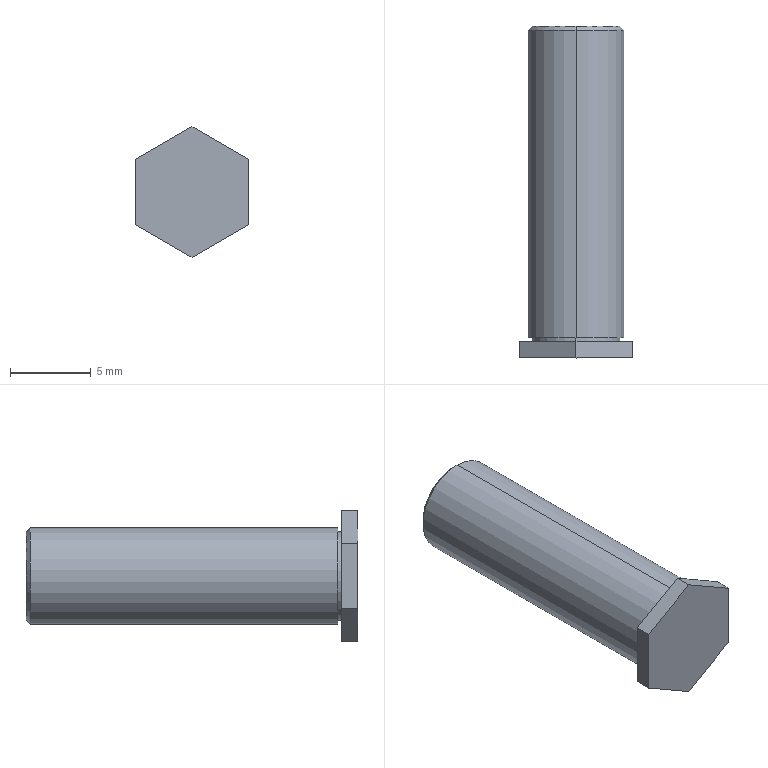Part | NX | features BREP 1 | 1 solid | 21 faces | box 7 x 20.5 x 8.083 mm | volume 432.929 mm3 | plane 11 | cylinder 6 | cone 4 | commonest cylinder face diameters 3.3 x2 5.45 x2 5.95 x2
STEP:
#1=CARTESIAN_POINT('',(300.5,41.65,424.025));
#2=VERTEX_POINT('',#1);
#3=CARTESIAN_POINT('',(300.5,41.65,429.975));
#4=VERTEX_POINT('',#3);
#5=CARTESIAN_POINT('',(300.5,41.65,427.));
#6=DIRECTION('',(0.,-1.,0.));
#7=DIRECTION('',(0.,0.,-1.));
#8=AXIS2_PLACEMENT_3D('',#5,#6,#7);
#9=CIRCLE('',#8,2.975);
#10=EDGE_CURVE('',#2,#4,#9,.T.);
#11=ORIENTED_EDGE('',*,*,#10,.T.);
#12=CARTESIAN_POINT('',(300.5,22.65,429.975));
#13=VERTEX_POINT('',#12);
#14=CARTESIAN_POINT('',(300.5,31.4,429.975));
#15=DIRECTION('',(0.,-1.,0.));
#16=VECTOR('',#15,1000.);
#17=LINE('',#14,#16);
#18=EDGE_CURVE('',#13,#4,#17,.F.);
#19=ORIENTED_EDGE('',*,*,#18,.F.);
#20=CARTESIAN_POINT('',(300.5,22.65,424.025));
#21=VERTEX_POINT('',#20);
#22=CARTESIAN_POINT('',(300.5,22.65,427.));
#23=DIRECTION('',(0.,1.,0.));
#24=DIRECTION('',(0.,0.,-1.));
#25=AXIS2_PLACEMENT_3D('',#22,#23,#24);
#26=CIRCLE('',#25,2.975);
#27=EDGE_CURVE('',#13,#21,#26,.T.);
#28=ORIENTED_EDGE('',*,*,#27,.T.);
#29=CARTESIAN_POINT('',(300.5,31.4,424.025));
#30=DIRECTION('',(0.,-1.,0.));
#31=VECTOR('',#30,1000.);
#32=LINE('',#29,#31);
#33=EDGE_CURVE('',#21,#2,#32,.F.);
#34=ORIENTED_EDGE('',*,*,#33,.T.);
#35=EDGE_LOOP('',(#11,#19,#28,#34));
#36=FACE_BOUND('',#35,.T.);
#37=CARTESIAN_POINT('',(300.5,31.4,427.));
#38=DIRECTION('',(0.,-1.,0.));
#39=DIRECTION('',(0.,0.,1.));
#40=AXIS2_PLACEMENT_3D('',#37,#38,#39);
#41=CYLINDRICAL_SURFACE('',#40,2.975);
#42=ADVANCED_FACE('',(#36),#41,.T.);
#43=CARTESIAN_POINT('',(300.5,41.9,424.275));
#44=VERTEX_POINT('',#43);
#45=CARTESIAN_POINT('',(300.5,41.9,429.725));
#46=VERTEX_POINT('',#45);
#47=CARTESIAN_POINT('',(300.5,41.9,427.));
#48=DIRECTION('',(0.,-1.,0.));
#49=DIRECTION('',(0.,0.,-1.));
#50=AXIS2_PLACEMENT_3D('',#47,#48,#49);
#51=CIRCLE('',#50,2.725);
#52=EDGE_CURVE('',#44,#46,#51,.T.);
#53=ORIENTED_EDGE('',*,*,#52,.T.);
#54=CARTESIAN_POINT('',(300.5,41.65,429.975));
#55=DIRECTION('',(0.,-0.7071,0.7071));
#56=VECTOR('',#55,1000.);
#57=LINE('',#54,#56);
#58=EDGE_CURVE('',#4,#46,#57,.F.);
#59=ORIENTED_EDGE('',*,*,#58,.F.);
#60=ORIENTED_EDGE('',*,*,#10,.F.);
#61=CARTESIAN_POINT('',(300.5,41.65,424.025));
#62=DIRECTION('',(0.,-0.7071,-0.7071));
#63=VECTOR('',#62,1000.);
#64=LINE('',#61,#63);
#65=EDGE_CURVE('',#2,#44,#64,.F.);
#66=ORIENTED_EDGE('',*,*,#65,.T.);
#67=EDGE_LOOP('',(#53,#59,#60,#66));
#68=FACE_BOUND('',#67,.T.);
#69=CARTESIAN_POINT('',(300.5,41.65,427.));
#70=DIRECTION('',(0.,-1.,0.));
#71=DIRECTION('',(0.,0.,1.));
#72=AXIS2_PLACEMENT_3D('',#69,#70,#71);
#73=CONICAL_SURFACE('',#72,2.975,0.7854);
#74=ADVANCED_FACE('',(#68),#73,.T.);
#75=CARTESIAN_POINT('',(300.5,22.4,429.725));
#76=VERTEX_POINT('',#75);
#77=CARTESIAN_POINT('',(300.5,22.4,424.275));
#78=VERTEX_POINT('',#77);
#79=CARTESIAN_POINT('',(300.5,22.4,427.));
#80=DIRECTION('',(0.,1.,0.));
#81=DIRECTION('',(0.,0.,1.));
#82=AXIS2_PLACEMENT_3D('',#79,#80,#81);
#83=CIRCLE('',#82,2.725);
#84=EDGE_CURVE('',#76,#78,#83,.T.);
#85=ORIENTED_EDGE('',*,*,#84,.T.);
#86=CARTESIAN_POINT('',(300.5,22.65,424.275));
#87=VERTEX_POINT('',#86);
#88=CARTESIAN_POINT('',(300.5,-1.133,424.275));
#89=DIRECTION('',(0.,1.,0.));
#90=VECTOR('',#89,1000.);
#91=LINE('',#88,#90);
#92=EDGE_CURVE('',#78,#87,#91,.T.);
#93=ORIENTED_EDGE('',*,*,#92,.T.);
#94=CARTESIAN_POINT('',(300.5,22.65,429.725));
#95=VERTEX_POINT('',#94);
#96=CARTESIAN_POINT('',(300.5,22.65,427.));
#97=DIRECTION('',(0.,-1.,0.));
#98=DIRECTION('',(0.,0.,1.));
#99=AXIS2_PLACEMENT_3D('',#96,#97,#98);
#100=CIRCLE('',#99,2.725);
#101=EDGE_CURVE('',#87,#95,#100,.T.);
#102=ORIENTED_EDGE('',*,*,#101,.T.);
#103=CARTESIAN_POINT('',(300.5,-1.133,429.725));
#104=DIRECTION('',(0.,1.,0.));
#105=VECTOR('',#104,1000.);
#106=LINE('',#103,#105);
#107=EDGE_CURVE('',#76,#95,#106,.T.);
#108=ORIENTED_EDGE('',*,*,#107,.F.);
#109=EDGE_LOOP('',(#85,#93,#102,#108));
#110=FACE_BOUND('',#109,.T.);
#111=CARTESIAN_POINT('',(300.5,-1.133,427.));
#112=DIRECTION('',(0.,1.,0.));
#113=DIRECTION('',(0.,0.,-1.));
#114=AXIS2_PLACEMENT_3D('',#111,#112,#113);
#115=CYLINDRICAL_SURFACE('',#114,2.725);
#116=ADVANCED_FACE('',(#110),#115,.T.);
#117=CARTESIAN_POINT('',(300.5,41.65,425.35));
#118=VERTEX_POINT('',#117);
#119=CARTESIAN_POINT('',(300.5,41.65,428.65));
#120=VERTEX_POINT('',#119);
#121=CARTESIAN_POINT('',(300.5,41.65,427.));
#122=DIRECTION('',(0.,1.,0.));
#123=DIRECTION('',(0.,0.,1.));
#124=AXIS2_PLACEMENT_3D('',#121,#122,#123);
#125=CIRCLE('',#124,1.65);
#126=EDGE_CURVE('',#118,#120,#125,.T.);
#127=ORIENTED_EDGE('',*,*,#126,.F.);
#128=CARTESIAN_POINT('',(300.5,41.9,425.1));
#129=VERTEX_POINT('',#128);
#130=CARTESIAN_POINT('',(300.5,41.9,425.1));
#131=DIRECTION('',(0.,0.7071,-0.7071));
#132=VECTOR('',#131,1000.);
#133=LINE('',#130,#132);
#134=EDGE_CURVE('',#118,#129,#133,.T.);
#135=ORIENTED_EDGE('',*,*,#134,.T.);
#136=CARTESIAN_POINT('',(300.5,41.9,428.9));
#137=VERTEX_POINT('',#136);
#138=CARTESIAN_POINT('',(300.5,41.9,427.));
#139=DIRECTION('',(0.,-1.,0.));
#140=DIRECTION('',(0.,0.,1.));
#141=AXIS2_PLACEMENT_3D('',#138,#139,#140);
#142=CIRCLE('',#141,1.9);
#143=EDGE_CURVE('',#137,#129,#142,.T.);
#144=ORIENTED_EDGE('',*,*,#143,.F.);
#145=CARTESIAN_POINT('',(300.5,41.9,428.9));
#146=DIRECTION('',(0.,0.7071,0.7071));
#147=VECTOR('',#146,1000.);
#148=LINE('',#145,#147);
#149=EDGE_CURVE('',#120,#137,#148,.T.);
#150=ORIENTED_EDGE('',*,*,#149,.F.);
#151=EDGE_LOOP('',(#127,#135,#144,#150));
#152=FACE_BOUND('',#151,.T.);
#153=CARTESIAN_POINT('',(300.5,41.9,427.));
#154=DIRECTION('',(0.,1.,0.));
#155=DIRECTION('',(0.,0.,-1.));
#156=AXIS2_PLACEMENT_3D('',#153,#154,#155);
#157=CONICAL_SURFACE('',#156,1.9,0.7854);
#158=ADVANCED_FACE('',(#152),#157,.F.);
#159=CARTESIAN_POINT('',(300.5,24.4,425.35));
#160=VERTEX_POINT('',#159);
#161=CARTESIAN_POINT('',(300.5,24.4,428.65));
#162=VERTEX_POINT('',#161);
#163=CARTESIAN_POINT('',(300.5,24.4,427.));
#164=DIRECTION('',(0.,1.,0.));
#165=DIRECTION('',(0.,0.,1.));
#166=AXIS2_PLACEMENT_3D('',#163,#164,#165);
#167=CIRCLE('',#166,1.65);
#168=EDGE_CURVE('',#160,#162,#167,.T.);
#169=ORIENTED_EDGE('',*,*,#168,.F.);
#170=CARTESIAN_POINT('',(300.5,24.4,425.35));
#171=DIRECTION('',(0.,1.,0.));
#172=VECTOR('',#171,1000.);
#173=LINE('',#170,#172);
#174=EDGE_CURVE('',#160,#118,#173,.T.);
#175=ORIENTED_EDGE('',*,*,#174,.T.);
#176=ORIENTED_EDGE('',*,*,#126,.T.);
#177=CARTESIAN_POINT('',(300.5,24.4,428.65));
#178=DIRECTION('',(0.,1.,0.));
#179=VECTOR('',#178,1000.);
#180=LINE('',#177,#179);
#181=EDGE_CURVE('',#162,#120,#180,.T.);
#182=ORIENTED_EDGE('',*,*,#181,.F.);
#183=EDGE_LOOP('',(#169,#175,#176,#182));
#184=FACE_BOUND('',#183,.T.);
#185=CARTESIAN_POINT('',(300.5,24.4,427.));
#186=DIRECTION('',(0.,1.,0.));
#187=DIRECTION('',(0.,0.,-1.));
#188=AXIS2_PLACEMENT_3D('',#185,#186,#187);
#189=CYLINDRICAL_SURFACE('',#188,1.65);
#190=ADVANCED_FACE('',(#184),#189,.F.);
#191=ORIENTED_EDGE('',*,*,#18,.T.);
#192=CARTESIAN_POINT('',(300.5,41.65,427.));
#193=DIRECTION('',(0.,-1.,0.));
#194=DIRECTION('',(0.,0.,-1.));
#195=AXIS2_PLACEMENT_3D('',#192,#193,#194);
#196=CIRCLE('',#195,2.975);
#197=EDGE_CURVE('',#4,#2,#196,.T.);
#198=ORIENTED_EDGE('',*,*,#197,.T.);
#199=ORIENTED_EDGE('',*,*,#33,.F.);
#200=CARTESIAN_POINT('',(300.5,22.65,427.));
#201=DIRECTION('',(0.,1.,0.));
#202=DIRECTION('',(0.,0.,-1.));
#203=AXIS2_PLACEMENT_3D('',#200,#201,#202);
#204=CIRCLE('',#203,2.975);
#205=EDGE_CURVE('',#21,#13,#204,.T.);
#206=ORIENTED_EDGE('',*,*,#205,.T.);
#207=EDGE_LOOP('',(#191,#198,#199,#206));
#208=FACE_BOUND('',#207,.T.);
#209=CARTESIAN_POINT('',(300.5,31.4,427.));
#210=DIRECTION('',(0.,-1.,0.));
#211=DIRECTION('',(0.,0.,1.));
#212=AXIS2_PLACEMENT_3D('',#209,#210,#211);
#213=CYLINDRICAL_SURFACE('',#212,2.975);
#214=ADVANCED_FACE('',(#208),#213,.T.);
#215=ORIENTED_EDGE('',*,*,#205,.F.);
#216=ORIENTED_EDGE('',*,*,#27,.F.);
#217=EDGE_LOOP('',(#215,#216));
#218=FACE_BOUND('',#217,.T.);
#219=CARTESIAN_POINT('',(300.5,22.65,427.));
#220=DIRECTION('',(0.,-1.,0.));
#221=DIRECTION('',(0.,0.,1.));
#222=AXIS2_PLACEMENT_3D('',#219,#220,#221);
#223=CIRCLE('',#222,2.725);
#224=EDGE_CURVE('',#95,#87,#223,.T.);
#225=ORIENTED_EDGE('',*,*,#224,.F.);
#226=ORIENTED_EDGE('',*,*,#101,.F.);
#227=EDGE_LOOP('',(#225,#226));
#228=FACE_BOUND('',#227,.T.);
#229=CARTESIAN_POINT('',(300.5,22.65,427.));
#230=DIRECTION('',(0.,1.,0.));
#231=DIRECTION('',(0.,0.,-1.));
#232=AXIS2_PLACEMENT_3D('',#229,#230,#231);
#233=PLANE('',#232);
#234=ADVANCED_FACE('',(#218,#228),#233,.F.);
#235=ORIENTED_EDGE('',*,*,#58,.T.);
#236=CARTESIAN_POINT('',(300.5,41.9,427.));
#237=DIRECTION('',(0.,-1.,0.));
#238=DIRECTION('',(0.,0.,-1.));
#239=AXIS2_PLACEMENT_3D('',#236,#237,#238);
#240=CIRCLE('',#239,2.725);
#241=EDGE_CURVE('',#46,#44,#240,.T.);
#242=ORIENTED_EDGE('',*,*,#241,.T.);
#243=ORIENTED_EDGE('',*,*,#65,.F.);
#244=ORIENTED_EDGE('',*,*,#197,.F.);
#245=EDGE_LOOP('',(#235,#242,#243,#244));
#246=FACE_BOUND('',#245,.T.);
#247=CARTESIAN_POINT('',(300.5,41.65,427.));
#248=DIRECTION('',(0.,-1.,0.));
#249=DIRECTION('',(0.,0.,1.));
#250=AXIS2_PLACEMENT_3D('',#247,#248,#249);
#251=CONICAL_SURFACE('',#250,2.975,0.7854);
#252=ADVANCED_FACE('',(#246),#251,.T.);
#253=ORIENTED_EDGE('',*,*,#92,.F.);
#254=CARTESIAN_POINT('',(300.5,22.4,427.));
#255=DIRECTION('',(0.,1.,0.));
#256=DIRECTION('',(0.,0.,1.));
#257=AXIS2_PLACEMENT_3D('',#254,#255,#256);
#258=CIRCLE('',#257,2.725);
#259=EDGE_CURVE('',#78,#76,#258,.T.);
#260=ORIENTED_EDGE('',*,*,#259,.T.);
#261=ORIENTED_EDGE('',*,*,#107,.T.);
#262=ORIENTED_EDGE('',*,*,#224,.T.);
#263=EDGE_LOOP('',(#253,#260,#261,#262));
#264=FACE_BOUND('',#263,.T.);
#265=CARTESIAN_POINT('',(300.5,-1.133,427.));
#266=DIRECTION('',(0.,1.,0.));
#267=DIRECTION('',(0.,0.,-1.));
#268=AXIS2_PLACEMENT_3D('',#265,#266,#267);
#269=CYLINDRICAL_SURFACE('',#268,2.725);
#270=ADVANCED_FACE('',(#264),#269,.T.);
#271=ORIENTED_EDGE('',*,*,#52,.F.);
#272=ORIENTED_EDGE('',*,*,#241,.F.);
#273=EDGE_LOOP('',(#271,#272));
#274=FACE_BOUND('',#273,.T.);
#275=ORIENTED_EDGE('',*,*,#143,.T.);
#276=CARTESIAN_POINT('',(300.5,41.9,427.));
#277=DIRECTION('',(0.,-1.,0.));
#278=DIRECTION('',(0.,0.,1.));
#279=AXIS2_PLACEMENT_3D('',#276,#277,#278);
#280=CIRCLE('',#279,1.9);
#281=EDGE_CURVE('',#129,#137,#280,.T.);
#282=ORIENTED_EDGE('',*,*,#281,.T.);
#283=EDGE_LOOP('',(#275,#282));
#284=FACE_BOUND('',#283,.T.);
#285=CARTESIAN_POINT('',(300.5,41.9,427.));
#286=DIRECTION('',(0.,1.,0.));
#287=DIRECTION('',(0.,0.,-1.));
#288=AXIS2_PLACEMENT_3D('',#285,#286,#287);
#289=PLANE('',#288);
#290=ADVANCED_FACE('',(#274,#284),#289,.T.);
#291=CARTESIAN_POINT('',(300.5,22.4,422.959));
#292=VERTEX_POINT('',#291);
#293=CARTESIAN_POINT('',(297.,22.4,424.979));
#294=VERTEX_POINT('',#293);
#295=CARTESIAN_POINT('',(300.5,22.4,422.959));
#296=DIRECTION('',(-0.866,0.,0.5));
#297=VECTOR('',#296,1000.);
#298=LINE('',#295,#297);
#299=EDGE_CURVE('',#292,#294,#298,.T.);
#300=ORIENTED_EDGE('',*,*,#299,.T.);
#301=CARTESIAN_POINT('',(297.,22.4,429.021));
#302=VERTEX_POINT('',#301);
#303=CARTESIAN_POINT('',(297.,22.4,427.));
#304=DIRECTION('',(0.,0.,1.));
#305=VECTOR('',#304,1000.);
#306=LINE('',#303,#305);
#307=EDGE_CURVE('',#294,#302,#306,.T.);
#308=ORIENTED_EDGE('',*,*,#307,.T.);
#309=CARTESIAN_POINT('',(300.5,22.4,431.041));
#310=VERTEX_POINT('',#309);
#311=CARTESIAN_POINT('',(297.,22.4,429.021));
#312=DIRECTION('',(0.866,0.,0.5));
#313=VECTOR('',#312,1000.);
#314=LINE('',#311,#313);
#315=EDGE_CURVE('',#302,#310,#314,.T.);
#316=ORIENTED_EDGE('',*,*,#315,.T.);
#317=CARTESIAN_POINT('',(304.,22.4,429.021));
#318=VERTEX_POINT('',#317);
#319=CARTESIAN_POINT('',(300.5,22.4,431.041));
#320=DIRECTION('',(0.866,0.,-0.5));
#321=VECTOR('',#320,1000.);
#322=LINE('',#319,#321);
#323=EDGE_CURVE('',#310,#318,#322,.T.);
#324=ORIENTED_EDGE('',*,*,#323,.T.);
#325=CARTESIAN_POINT('',(304.,22.4,424.979));
#326=VERTEX_POINT('',#325);
#327=CARTESIAN_POINT('',(304.,22.4,427.));
#328=DIRECTION('',(0.,0.,-1.));
#329=VECTOR('',#328,1000.);
#330=LINE('',#327,#329);
#331=EDGE_CURVE('',#318,#326,#330,.T.);
#332=ORIENTED_EDGE('',*,*,#331,.T.);
#333=CARTESIAN_POINT('',(304.,22.4,424.979));
#334=DIRECTION('',(-0.866,0.,-0.5));
#335=VECTOR('',#334,1000.);
#336=LINE('',#333,#335);
#337=EDGE_CURVE('',#326,#292,#336,.T.);
#338=ORIENTED_EDGE('',*,*,#337,.T.);
#339=EDGE_LOOP('',(#300,#308,#316,#324,#332,#338));
#340=FACE_BOUND('',#339,.T.);
#341=ORIENTED_EDGE('',*,*,#84,.F.);
#342=ORIENTED_EDGE('',*,*,#259,.F.);
#343=EDGE_LOOP('',(#341,#342));
#344=FACE_BOUND('',#343,.T.);
#345=CARTESIAN_POINT('',(300.5,22.4,427.));
#346=DIRECTION('',(0.,1.,0.));
#347=DIRECTION('',(0.,0.,-1.));
#348=AXIS2_PLACEMENT_3D('',#345,#346,#347);
#349=PLANE('',#348);
#350=ADVANCED_FACE('',(#340,#344),#349,.T.);
#351=ORIENTED_EDGE('',*,*,#134,.F.);
#352=CARTESIAN_POINT('',(300.5,41.65,427.));
#353=DIRECTION('',(0.,1.,0.));
#354=DIRECTION('',(0.,0.,1.));
#355=AXIS2_PLACEMENT_3D('',#352,#353,#354);
#356=CIRCLE('',#355,1.65);
#357=EDGE_CURVE('',#120,#118,#356,.T.);
#358=ORIENTED_EDGE('',*,*,#357,.F.);
#359=ORIENTED_EDGE('',*,*,#149,.T.);
#360=ORIENTED_EDGE('',*,*,#281,.F.);
#361=EDGE_LOOP('',(#351,#358,#359,#360));
#362=FACE_BOUND('',#361,.T.);
#363=CARTESIAN_POINT('',(300.5,41.9,427.));
#364=DIRECTION('',(0.,1.,0.));
#365=DIRECTION('',(0.,0.,-1.));
#366=AXIS2_PLACEMENT_3D('',#363,#364,#365);
#367=CONICAL_SURFACE('',#366,1.9,0.7854);
#368=ADVANCED_FACE('',(#362),#367,.F.);
#369=CARTESIAN_POINT('',(297.,21.4,424.979));
#370=VERTEX_POINT('',#369);
#371=CARTESIAN_POINT('',(297.,22.4,424.979));
#372=DIRECTION('',(0.,1.,0.));
#373=VECTOR('',#372,1000.);
#374=LINE('',#371,#373);
#375=EDGE_CURVE('',#370,#294,#374,.T.);
#376=ORIENTED_EDGE('',*,*,#375,.F.);
#377=CARTESIAN_POINT('',(297.,21.4,429.021));
#378=VERTEX_POINT('',#377);
#379=CARTESIAN_POINT('',(297.,21.4,424.979));
#380=DIRECTION('',(0.,0.,-1.));
#381=VECTOR('',#380,1000.);
#382=LINE('',#379,#381);
#383=EDGE_CURVE('',#378,#370,#382,.T.);
#384=ORIENTED_EDGE('',*,*,#383,.F.);
#385=CARTESIAN_POINT('',(297.,22.4,429.021));
#386=DIRECTION('',(0.,-1.,0.));
#387=VECTOR('',#386,1000.);
#388=LINE('',#385,#387);
#389=EDGE_CURVE('',#302,#378,#388,.T.);
#390=ORIENTED_EDGE('',*,*,#389,.F.);
#391=ORIENTED_EDGE('',*,*,#307,.F.);
#392=EDGE_LOOP('',(#376,#384,#390,#391));
#393=FACE_BOUND('',#392,.T.);
#394=CARTESIAN_POINT('',(297.,22.4,424.979));
#395=DIRECTION('',(1.,0.,0.));
#396=DIRECTION('',(0.,0.,1.));
#397=AXIS2_PLACEMENT_3D('',#394,#395,#396);
#398=PLANE('',#397);
#399=ADVANCED_FACE('',(#393),#398,.F.);
#400=CARTESIAN_POINT('',(300.5,21.4,422.959));
#401=VERTEX_POINT('',#400);
#402=CARTESIAN_POINT('',(300.5,22.4,422.959));
#403=DIRECTION('',(0.,1.,0.));
#404=VECTOR('',#403,1000.);
#405=LINE('',#402,#404);
#406=EDGE_CURVE('',#401,#292,#405,.T.);
#407=ORIENTED_EDGE('',*,*,#406,.F.);
#408=CARTESIAN_POINT('',(300.5,21.4,422.959));
#409=DIRECTION('',(0.866,0.,-0.5));
#410=VECTOR('',#409,1000.);
#411=LINE('',#408,#410);
#412=EDGE_CURVE('',#370,#401,#411,.T.);
#413=ORIENTED_EDGE('',*,*,#412,.F.);
#414=ORIENTED_EDGE('',*,*,#375,.T.);
#415=ORIENTED_EDGE('',*,*,#299,.F.);
#416=EDGE_LOOP('',(#407,#413,#414,#415));
#417=FACE_BOUND('',#416,.T.);
#418=CARTESIAN_POINT('',(300.5,22.4,422.959));
#419=DIRECTION('',(0.5,0.,0.866));
#420=DIRECTION('',(-0.866,0.,0.5));
#421=AXIS2_PLACEMENT_3D('',#418,#419,#420);
#422=PLANE('',#421);
#423=ADVANCED_FACE('',(#417),#422,.F.);
#424=CARTESIAN_POINT('',(304.,21.4,424.979));
#425=VERTEX_POINT('',#424);
#426=CARTESIAN_POINT('',(304.,22.4,424.979));
#427=DIRECTION('',(0.,1.,0.));
#428=VECTOR('',#427,1000.);
#429=LINE('',#426,#428);
#430=EDGE_CURVE('',#425,#326,#429,.T.);
#431=ORIENTED_EDGE('',*,*,#430,.F.);
#432=CARTESIAN_POINT('',(304.,21.4,424.979));
#433=DIRECTION('',(0.866,0.,0.5));
#434=VECTOR('',#433,1000.);
#435=LINE('',#432,#434);
#436=EDGE_CURVE('',#401,#425,#435,.T.);
#437=ORIENTED_EDGE('',*,*,#436,.F.);
#438=ORIENTED_EDGE('',*,*,#406,.T.);
#439=ORIENTED_EDGE('',*,*,#337,.F.);
#440=EDGE_LOOP('',(#431,#437,#438,#439));
#441=FACE_BOUND('',#440,.T.);
#442=CARTESIAN_POINT('',(304.,22.4,424.979));
#443=DIRECTION('',(-0.5,0.,0.866));
#444=DIRECTION('',(-0.866,0.,-0.5));
#445=AXIS2_PLACEMENT_3D('',#442,#443,#444);
#446=PLANE('',#445);
#447=ADVANCED_FACE('',(#441),#446,.F.);
#448=CARTESIAN_POINT('',(304.,21.4,429.021));
#449=VERTEX_POINT('',#448);
#450=CARTESIAN_POINT('',(304.,22.4,429.021));
#451=DIRECTION('',(0.,1.,0.));
#452=VECTOR('',#451,1000.);
#453=LINE('',#450,#452);
#454=EDGE_CURVE('',#449,#318,#453,.T.);
#455=ORIENTED_EDGE('',*,*,#454,.F.);
#456=CARTESIAN_POINT('',(304.,21.4,429.021));
#457=DIRECTION('',(0.,0.,1.));
#458=VECTOR('',#457,1000.);
#459=LINE('',#456,#458);
#460=EDGE_CURVE('',#425,#449,#459,.T.);
#461=ORIENTED_EDGE('',*,*,#460,.F.);
#462=ORIENTED_EDGE('',*,*,#430,.T.);
#463=ORIENTED_EDGE('',*,*,#331,.F.);
#464=EDGE_LOOP('',(#455,#461,#462,#463));
#465=FACE_BOUND('',#464,.T.);
#466=CARTESIAN_POINT('',(304.,22.4,429.021));
#467=DIRECTION('',(-1.,0.,0.));
#468=DIRECTION('',(0.,0.,-1.));
#469=AXIS2_PLACEMENT_3D('',#466,#467,#468);
#470=PLANE('',#469);
#471=ADVANCED_FACE('',(#465),#470,.F.);
#472=CARTESIAN_POINT('',(300.5,21.4,431.041));
#473=VERTEX_POINT('',#472);
#474=CARTESIAN_POINT('',(300.5,22.4,431.041));
#475=DIRECTION('',(0.,1.,0.));
#476=VECTOR('',#475,1000.);
#477=LINE('',#474,#476);
#478=EDGE_CURVE('',#473,#310,#477,.T.);
#479=ORIENTED_EDGE('',*,*,#478,.F.);
#480=CARTESIAN_POINT('',(300.5,21.4,431.041));
#481=DIRECTION('',(-0.866,0.,0.5));
#482=VECTOR('',#481,1000.);
#483=LINE('',#480,#482);
#484=EDGE_CURVE('',#449,#473,#483,.T.);
#485=ORIENTED_EDGE('',*,*,#484,.F.);
#486=ORIENTED_EDGE('',*,*,#454,.T.);
#487=ORIENTED_EDGE('',*,*,#323,.F.);
#488=EDGE_LOOP('',(#479,#485,#486,#487));
#489=FACE_BOUND('',#488,.T.);
#490=CARTESIAN_POINT('',(300.5,22.4,431.041));
#491=DIRECTION('',(-0.5,0.,-0.866));
#492=DIRECTION('',(0.866,0.,-0.5));
#493=AXIS2_PLACEMENT_3D('',#490,#491,#492);
#494=PLANE('',#493);
#495=ADVANCED_FACE('',(#489),#494,.F.);
#496=ORIENTED_EDGE('',*,*,#389,.T.);
#497=CARTESIAN_POINT('',(297.,21.4,429.021));
#498=DIRECTION('',(-0.866,0.,-0.5));
#499=VECTOR('',#498,1000.);
#500=LINE('',#497,#499);
#501=EDGE_CURVE('',#473,#378,#500,.T.);
#502=ORIENTED_EDGE('',*,*,#501,.F.);
#503=ORIENTED_EDGE('',*,*,#478,.T.);
#504=ORIENTED_EDGE('',*,*,#315,.F.);
#505=EDGE_LOOP('',(#496,#502,#503,#504));
#506=FACE_BOUND('',#505,.T.);
#507=CARTESIAN_POINT('',(297.,22.4,429.021));
#508=DIRECTION('',(0.5,0.,-0.866));
#509=DIRECTION('',(0.866,0.,0.5));
#510=AXIS2_PLACEMENT_3D('',#507,#508,#509);
#511=PLANE('',#510);
#512=ADVANCED_FACE('',(#506),#511,.F.);
#513=ORIENTED_EDGE('',*,*,#174,.F.);
#514=CARTESIAN_POINT('',(300.5,24.4,427.));
#515=DIRECTION('',(0.,1.,0.));
#516=DIRECTION('',(0.,0.,1.));
#517=AXIS2_PLACEMENT_3D('',#514,#515,#516);
#518=CIRCLE('',#517,1.65);
#519=EDGE_CURVE('',#162,#160,#518,.T.);
#520=ORIENTED_EDGE('',*,*,#519,.F.);
#521=ORIENTED_EDGE('',*,*,#181,.T.);
#522=ORIENTED_EDGE('',*,*,#357,.T.);
#523=EDGE_LOOP('',(#513,#520,#521,#522));
#524=FACE_BOUND('',#523,.T.);
#525=CARTESIAN_POINT('',(300.5,24.4,427.));
#526=DIRECTION('',(0.,1.,0.));
#527=DIRECTION('',(0.,0.,-1.));
#528=AXIS2_PLACEMENT_3D('',#525,#526,#527);
#529=CYLINDRICAL_SURFACE('',#528,1.65);
#530=ADVANCED_FACE('',(#524),#529,.F.);
#531=ORIENTED_EDGE('',*,*,#460,.T.);
#532=ORIENTED_EDGE('',*,*,#484,.T.);
#533=ORIENTED_EDGE('',*,*,#501,.T.);
#534=ORIENTED_EDGE('',*,*,#383,.T.);
#535=ORIENTED_EDGE('',*,*,#412,.T.);
#536=ORIENTED_EDGE('',*,*,#436,.T.);
#537=EDGE_LOOP('',(#531,#532,#533,#534,#535,#536));
#538=FACE_BOUND('',#537,.T.);
#539=CARTESIAN_POINT('',(300.5,21.4,427.));
#540=DIRECTION('',(0.,1.,0.));
#541=DIRECTION('',(0.,0.,-1.));
#542=AXIS2_PLACEMENT_3D('',#539,#540,#541);
#543=PLANE('',#542);
#544=ADVANCED_FACE('',(#538),#543,.F.);
#545=ORIENTED_EDGE('',*,*,#519,.T.);
#546=ORIENTED_EDGE('',*,*,#168,.T.);
#547=EDGE_LOOP('',(#545,#546));
#548=FACE_BOUND('',#547,.T.);
#549=CARTESIAN_POINT('',(300.5,24.4,427.));
#550=DIRECTION('',(0.,1.,0.));
#551=DIRECTION('',(0.,0.,-1.));
#552=AXIS2_PLACEMENT_3D('',#549,#550,#551);
#553=PLANE('',#552);
#554=ADVANCED_FACE('',(#548),#553,.T.);
#555=CLOSED_SHELL('',(#42,#74,#116,#158,#190,#214,#234,#252,#270,#290,#350,#368,#399,#423,#447,#471,#495,#512,#530,#544,#554));
#556=MANIFOLD_SOLID_BREP('',#555);
#557=(LENGTH_UNIT()NAMED_UNIT(*)SI_UNIT(.MILLI.,.METRE.));
#558=UNCERTAINTY_MEASURE_WITH_UNIT(LENGTH_MEASURE(0.00001),#557,'','');
#559=(NAMED_UNIT(*)PLANE_ANGLE_UNIT()SI_UNIT($,.RADIAN.));
#560=(NAMED_UNIT(*)SI_UNIT($,.STERADIAN.)SOLID_ANGLE_UNIT());
#561=(GEOMETRIC_REPRESENTATION_CONTEXT(3)GLOBAL_UNCERTAINTY_ASSIGNED_CONTEXT((#558))GLOBAL_UNIT_ASSIGNED_CONTEXT((#557,#559,#560))REPRESENTATION_CONTEXT('',''));
#562=ADVANCED_BREP_SHAPE_REPRESENTATION('',(#556),#561);